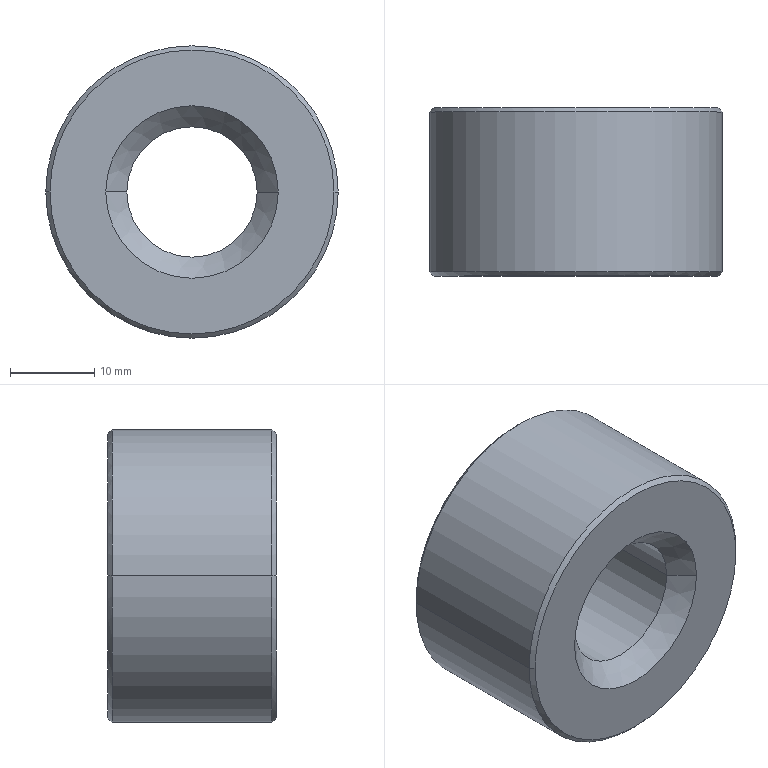Part | STEP file | CIHUAN_7_1 | 1 solid | 14 faces | box 34.75 x 20 x 34.75 mm | volume 14830 mm3 | cone 8 | cylinder 4 | plane 2 | commonest cylinder face diameters 15.5 x2 34.75 x2
STEP:
#1=CARTESIAN_POINT('',(0.,0.,0.));
#2=DIRECTION('',(0.,0.,1.));
#3=DIRECTION('',(1.,0.,0.));
#4=AXIS2_PLACEMENT_3D('',#1,#2,#3);
#5=CARTESIAN_POINT('',(16.875,0.,0.));
#6=VERTEX_POINT('',#5);
#7=CARTESIAN_POINT('',(0.,0.,-16.875));
#8=VERTEX_POINT('',#7);
#9=CARTESIAN_POINT('',(0.,0.,0.));
#10=DIRECTION('',(0.,1.,0.));
#11=DIRECTION('',(1.,0.,0.));
#12=AXIS2_PLACEMENT_3D('',#9,#10,#11);
#13=CIRCLE('',#12,16.875);
#14=EDGE_CURVE('',#6,#8,#13,.T.);
#15=ORIENTED_EDGE('',*,*,#14,.T.);
#16=CARTESIAN_POINT('',(-16.875,0.,0.));
#17=VERTEX_POINT('',#16);
#18=CARTESIAN_POINT('',(0.,0.,0.));
#19=DIRECTION('',(0.,1.,0.));
#20=DIRECTION('',(0.,0.,-1.));
#21=AXIS2_PLACEMENT_3D('',#18,#19,#20);
#22=CIRCLE('',#21,16.875);
#23=EDGE_CURVE('',#8,#17,#22,.T.);
#24=ORIENTED_EDGE('',*,*,#23,.T.);
#25=CARTESIAN_POINT('',(0.,0.,16.875));
#26=VERTEX_POINT('',#25);
#27=CARTESIAN_POINT('',(0.,0.,0.));
#28=DIRECTION('',(0.,1.,0.));
#29=DIRECTION('',(-1.,0.,0.));
#30=AXIS2_PLACEMENT_3D('',#27,#28,#29);
#31=CIRCLE('',#30,16.875);
#32=EDGE_CURVE('',#17,#26,#31,.T.);
#33=ORIENTED_EDGE('',*,*,#32,.T.);
#34=CARTESIAN_POINT('',(0.,0.,0.));
#35=DIRECTION('',(0.,1.,0.));
#36=DIRECTION('',(0.,0.,1.));
#37=AXIS2_PLACEMENT_3D('',#34,#35,#36);
#38=CIRCLE('',#37,16.875);
#39=EDGE_CURVE('',#26,#6,#38,.T.);
#40=ORIENTED_EDGE('',*,*,#39,.T.);
#41=EDGE_LOOP('',(#15,#24,#33,#40));
#42=FACE_OUTER_BOUND('',#41,.F.);
#43=CARTESIAN_POINT('',(-10.25,0.,0.));
#44=VERTEX_POINT('',#43);
#45=CARTESIAN_POINT('',(0.,0.,-10.25));
#46=VERTEX_POINT('',#45);
#47=CARTESIAN_POINT('',(0.,0.,0.));
#48=DIRECTION('',(0.,-1.,0.));
#49=DIRECTION('',(-1.,0.,0.));
#50=AXIS2_PLACEMENT_3D('',#47,#48,#49);
#51=CIRCLE('',#50,10.25);
#52=EDGE_CURVE('',#44,#46,#51,.T.);
#53=ORIENTED_EDGE('',*,*,#52,.T.);
#54=CARTESIAN_POINT('',(10.25,0.,0.));
#55=VERTEX_POINT('',#54);
#56=CARTESIAN_POINT('',(0.,0.,0.));
#57=DIRECTION('',(0.,-1.,0.));
#58=DIRECTION('',(0.,0.,-1.));
#59=AXIS2_PLACEMENT_3D('',#56,#57,#58);
#60=CIRCLE('',#59,10.25);
#61=EDGE_CURVE('',#46,#55,#60,.T.);
#62=ORIENTED_EDGE('',*,*,#61,.T.);
#63=CARTESIAN_POINT('',(0.,0.,10.25));
#64=VERTEX_POINT('',#63);
#65=CARTESIAN_POINT('',(0.,0.,0.));
#66=DIRECTION('',(0.,-1.,0.));
#67=DIRECTION('',(1.,0.,0.));
#68=AXIS2_PLACEMENT_3D('',#65,#66,#67);
#69=CIRCLE('',#68,10.25);
#70=EDGE_CURVE('',#55,#64,#69,.T.);
#71=ORIENTED_EDGE('',*,*,#70,.T.);
#72=CARTESIAN_POINT('',(0.,0.,0.));
#73=DIRECTION('',(0.,-1.,0.));
#74=DIRECTION('',(0.,0.,1.));
#75=AXIS2_PLACEMENT_3D('',#72,#73,#74);
#76=CIRCLE('',#75,10.25);
#77=EDGE_CURVE('',#64,#44,#76,.T.);
#78=ORIENTED_EDGE('',*,*,#77,.T.);
#79=EDGE_LOOP('',(#53,#62,#71,#78));
#80=FACE_BOUND('',#79,.F.);
#81=CARTESIAN_POINT('',(0.,0.,0.));
#82=DIRECTION('',(0.,1.,0.));
#83=DIRECTION('',(1.,0.,0.));
#84=AXIS2_PLACEMENT_3D('',#81,#82,#83);
#85=PLANE('',#84);
#86=ADVANCED_FACE('',(#42,#80),#85,.F.);
#87=ORIENTED_EDGE('',*,*,#23,.F.);
#88=ORIENTED_EDGE('',*,*,#14,.F.);
#89=CARTESIAN_POINT('',(17.375,0.5,-0.000000001));
#90=VERTEX_POINT('',#89);
#91=CARTESIAN_POINT('',(16.875,0.,-0.000000001));
#92=DIRECTION('',(0.7071,0.7071,0.));
#93=VECTOR('',#92,0.7071);
#94=LINE('',#91,#93);
#95=EDGE_CURVE('',#6,#90,#94,.T.);
#96=ORIENTED_EDGE('',*,*,#95,.T.);
#97=CARTESIAN_POINT('',(0.,0.5,-17.375));
#98=VERTEX_POINT('',#97);
#99=CARTESIAN_POINT('',(0.,0.5,0.));
#100=DIRECTION('',(0.,1.,0.));
#101=DIRECTION('',(1.,0.,0.));
#102=AXIS2_PLACEMENT_3D('',#99,#100,#101);
#103=CIRCLE('',#102,17.375);
#104=EDGE_CURVE('',#90,#98,#103,.T.);
#105=ORIENTED_EDGE('',*,*,#104,.T.);
#106=CARTESIAN_POINT('',(-17.375,0.5,0.000000002));
#107=VERTEX_POINT('',#106);
#108=CARTESIAN_POINT('',(0.,0.5,0.));
#109=DIRECTION('',(0.,1.,0.));
#110=DIRECTION('',(0.,0.,-1.));
#111=AXIS2_PLACEMENT_3D('',#108,#109,#110);
#112=CIRCLE('',#111,17.375);
#113=EDGE_CURVE('',#98,#107,#112,.T.);
#114=ORIENTED_EDGE('',*,*,#113,.T.);
#115=CARTESIAN_POINT('',(-16.875,0.,0.000000001));
#116=DIRECTION('',(-0.7071,0.7071,0.000000001));
#117=VECTOR('',#116,0.7071);
#118=LINE('',#115,#117);
#119=EDGE_CURVE('',#17,#107,#118,.T.);
#120=ORIENTED_EDGE('',*,*,#119,.F.);
#121=EDGE_LOOP('',(#87,#88,#96,#105,#114,#120));
#122=FACE_OUTER_BOUND('',#121,.F.);
#123=CARTESIAN_POINT('',(0.,0.25,0.));
#124=DIRECTION('',(0.,1.,0.));
#125=DIRECTION('',(0.,0.,-1.));
#126=AXIS2_PLACEMENT_3D('',#123,#124,#125);
#127=CONICAL_SURFACE('',#126,17.125,45.);
#128=ADVANCED_FACE('',(#122),#127,.T.);
#129=ORIENTED_EDGE('',*,*,#39,.F.);
#130=ORIENTED_EDGE('',*,*,#32,.F.);
#131=ORIENTED_EDGE('',*,*,#119,.T.);
#132=CARTESIAN_POINT('',(0.,0.5,17.375));
#133=VERTEX_POINT('',#132);
#134=CARTESIAN_POINT('',(0.,0.5,0.));
#135=DIRECTION('',(0.,1.,0.));
#136=DIRECTION('',(-1.,0.,0.));
#137=AXIS2_PLACEMENT_3D('',#134,#135,#136);
#138=CIRCLE('',#137,17.375);
#139=EDGE_CURVE('',#107,#133,#138,.T.);
#140=ORIENTED_EDGE('',*,*,#139,.T.);
#141=CARTESIAN_POINT('',(0.,0.5,0.));
#142=DIRECTION('',(0.,1.,0.));
#143=DIRECTION('',(0.,0.,1.));
#144=AXIS2_PLACEMENT_3D('',#141,#142,#143);
#145=CIRCLE('',#144,17.375);
#146=EDGE_CURVE('',#133,#90,#145,.T.);
#147=ORIENTED_EDGE('',*,*,#146,.T.);
#148=ORIENTED_EDGE('',*,*,#95,.F.);
#149=EDGE_LOOP('',(#129,#130,#131,#140,#147,#148));
#150=FACE_OUTER_BOUND('',#149,.F.);
#151=CARTESIAN_POINT('',(0.,0.25,0.));
#152=DIRECTION('',(0.,1.,0.));
#153=DIRECTION('',(0.,0.,-1.));
#154=AXIS2_PLACEMENT_3D('',#151,#152,#153);
#155=CONICAL_SURFACE('',#154,17.125,45.);
#156=ADVANCED_FACE('',(#150),#155,.T.);
#157=CARTESIAN_POINT('',(0.,19.5,17.375));
#158=VERTEX_POINT('',#157);
#159=CARTESIAN_POINT('',(-17.375,19.5,0.000000002));
#160=VERTEX_POINT('',#159);
#161=CARTESIAN_POINT('',(0.,19.5,0.));
#162=DIRECTION('',(0.,-1.,0.));
#163=DIRECTION('',(0.,0.,1.));
#164=AXIS2_PLACEMENT_3D('',#161,#162,#163);
#165=CIRCLE('',#164,17.375);
#166=EDGE_CURVE('',#158,#160,#165,.T.);
#167=ORIENTED_EDGE('',*,*,#166,.F.);
#168=CARTESIAN_POINT('',(17.375,19.5,0.));
#169=VERTEX_POINT('',#168);
#170=CARTESIAN_POINT('',(0.,19.5,0.));
#171=DIRECTION('',(0.,-1.,0.));
#172=DIRECTION('',(1.,0.,0.));
#173=AXIS2_PLACEMENT_3D('',#170,#171,#172);
#174=CIRCLE('',#173,17.375);
#175=EDGE_CURVE('',#169,#158,#174,.T.);
#176=ORIENTED_EDGE('',*,*,#175,.F.);
#177=CARTESIAN_POINT('',(17.375,0.5,-0.000000001));
#178=DIRECTION('',(0.,1.,0.));
#179=VECTOR('',#178,19.);
#180=LINE('',#177,#179);
#181=EDGE_CURVE('',#90,#169,#180,.T.);
#182=ORIENTED_EDGE('',*,*,#181,.F.);
#183=ORIENTED_EDGE('',*,*,#146,.F.);
#184=ORIENTED_EDGE('',*,*,#139,.F.);
#185=CARTESIAN_POINT('',(-17.375,0.5,0.000000002));
#186=DIRECTION('',(0.,1.,0.));
#187=VECTOR('',#186,19.);
#188=LINE('',#185,#187);
#189=EDGE_CURVE('',#107,#160,#188,.T.);
#190=ORIENTED_EDGE('',*,*,#189,.T.);
#191=EDGE_LOOP('',(#167,#176,#182,#183,#184,#190));
#192=FACE_OUTER_BOUND('',#191,.F.);
#193=CARTESIAN_POINT('',(0.,0.,0.));
#194=DIRECTION('',(0.,1.,0.));
#195=DIRECTION('',(1.,0.,0.));
#196=AXIS2_PLACEMENT_3D('',#193,#194,#195);
#197=CYLINDRICAL_SURFACE('',#196,17.375);
#198=ADVANCED_FACE('',(#192),#197,.T.);
#199=CARTESIAN_POINT('',(0.,20.,16.875));
#200=VERTEX_POINT('',#199);
#201=CARTESIAN_POINT('',(-16.875,20.,0.));
#202=VERTEX_POINT('',#201);
#203=CARTESIAN_POINT('',(0.,20.,0.));
#204=DIRECTION('',(0.,-1.,0.));
#205=DIRECTION('',(0.,0.,1.));
#206=AXIS2_PLACEMENT_3D('',#203,#204,#205);
#207=CIRCLE('',#206,16.875);
#208=EDGE_CURVE('',#200,#202,#207,.T.);
#209=ORIENTED_EDGE('',*,*,#208,.F.);
#210=CARTESIAN_POINT('',(16.875,20.,0.));
#211=VERTEX_POINT('',#210);
#212=CARTESIAN_POINT('',(0.,20.,0.));
#213=DIRECTION('',(0.,-1.,0.));
#214=DIRECTION('',(1.,0.,0.));
#215=AXIS2_PLACEMENT_3D('',#212,#213,#214);
#216=CIRCLE('',#215,16.875);
#217=EDGE_CURVE('',#211,#200,#216,.T.);
#218=ORIENTED_EDGE('',*,*,#217,.F.);
#219=CARTESIAN_POINT('',(16.875,20.,-0.000000001));
#220=DIRECTION('',(0.7071,-0.7071,0.));
#221=VECTOR('',#220,0.7071);
#222=LINE('',#219,#221);
#223=EDGE_CURVE('',#211,#169,#222,.T.);
#224=ORIENTED_EDGE('',*,*,#223,.T.);
#225=ORIENTED_EDGE('',*,*,#175,.T.);
#226=ORIENTED_EDGE('',*,*,#166,.T.);
#227=CARTESIAN_POINT('',(-16.875,20.,0.000000001));
#228=DIRECTION('',(-0.7071,-0.7071,0.000000001));
#229=VECTOR('',#228,0.7071);
#230=LINE('',#227,#229);
#231=EDGE_CURVE('',#202,#160,#230,.T.);
#232=ORIENTED_EDGE('',*,*,#231,.F.);
#233=EDGE_LOOP('',(#209,#218,#224,#225,#226,#232));
#234=FACE_OUTER_BOUND('',#233,.F.);
#235=CARTESIAN_POINT('',(0.,19.75,0.));
#236=DIRECTION('',(0.,-1.,0.));
#237=DIRECTION('',(0.,0.,-1.));
#238=AXIS2_PLACEMENT_3D('',#235,#236,#237);
#239=CONICAL_SURFACE('',#238,17.125,45.);
#240=ADVANCED_FACE('',(#234),#239,.T.);
#241=CARTESIAN_POINT('',(0.,20.,-16.875));
#242=VERTEX_POINT('',#241);
#243=CARTESIAN_POINT('',(0.,20.,0.));
#244=DIRECTION('',(0.,-1.,0.));
#245=DIRECTION('',(-1.,0.,0.));
#246=AXIS2_PLACEMENT_3D('',#243,#244,#245);
#247=CIRCLE('',#246,16.875);
#248=EDGE_CURVE('',#202,#242,#247,.T.);
#249=ORIENTED_EDGE('',*,*,#248,.T.);
#250=CARTESIAN_POINT('',(0.,20.,0.));
#251=DIRECTION('',(0.,-1.,0.));
#252=DIRECTION('',(0.,0.,-1.));
#253=AXIS2_PLACEMENT_3D('',#250,#251,#252);
#254=CIRCLE('',#253,16.875);
#255=EDGE_CURVE('',#242,#211,#254,.T.);
#256=ORIENTED_EDGE('',*,*,#255,.T.);
#257=ORIENTED_EDGE('',*,*,#217,.T.);
#258=ORIENTED_EDGE('',*,*,#208,.T.);
#259=EDGE_LOOP('',(#249,#256,#257,#258));
#260=FACE_OUTER_BOUND('',#259,.F.);
#261=CARTESIAN_POINT('',(10.25,20.,0.));
#262=VERTEX_POINT('',#261);
#263=CARTESIAN_POINT('',(0.,20.,-10.25));
#264=VERTEX_POINT('',#263);
#265=CARTESIAN_POINT('',(0.,20.,0.));
#266=DIRECTION('',(0.,1.,0.));
#267=DIRECTION('',(1.,0.,0.));
#268=AXIS2_PLACEMENT_3D('',#265,#266,#267);
#269=CIRCLE('',#268,10.25);
#270=EDGE_CURVE('',#262,#264,#269,.T.);
#271=ORIENTED_EDGE('',*,*,#270,.T.);
#272=CARTESIAN_POINT('',(-10.25,20.,0.));
#273=VERTEX_POINT('',#272);
#274=CARTESIAN_POINT('',(0.,20.,0.));
#275=DIRECTION('',(0.,1.,0.));
#276=DIRECTION('',(0.,0.,-1.));
#277=AXIS2_PLACEMENT_3D('',#274,#275,#276);
#278=CIRCLE('',#277,10.25);
#279=EDGE_CURVE('',#264,#273,#278,.T.);
#280=ORIENTED_EDGE('',*,*,#279,.T.);
#281=CARTESIAN_POINT('',(0.,20.,10.25));
#282=VERTEX_POINT('',#281);
#283=CARTESIAN_POINT('',(0.,20.,0.));
#284=DIRECTION('',(0.,1.,0.));
#285=DIRECTION('',(-1.,0.,0.));
#286=AXIS2_PLACEMENT_3D('',#283,#284,#285);
#287=CIRCLE('',#286,10.25);
#288=EDGE_CURVE('',#273,#282,#287,.T.);
#289=ORIENTED_EDGE('',*,*,#288,.T.);
#290=CARTESIAN_POINT('',(0.,20.,0.));
#291=DIRECTION('',(0.,1.,0.));
#292=DIRECTION('',(0.,0.,1.));
#293=AXIS2_PLACEMENT_3D('',#290,#291,#292);
#294=CIRCLE('',#293,10.25);
#295=EDGE_CURVE('',#282,#262,#294,.T.);
#296=ORIENTED_EDGE('',*,*,#295,.T.);
#297=EDGE_LOOP('',(#271,#280,#289,#296));
#298=FACE_BOUND('',#297,.F.);
#299=CARTESIAN_POINT('',(0.,20.,0.));
#300=DIRECTION('',(0.,1.,0.));
#301=DIRECTION('',(1.,0.,0.));
#302=AXIS2_PLACEMENT_3D('',#299,#300,#301);
#303=PLANE('',#302);
#304=ADVANCED_FACE('',(#260,#298),#303,.T.);
#305=ORIENTED_EDGE('',*,*,#255,.F.);
#306=ORIENTED_EDGE('',*,*,#248,.F.);
#307=ORIENTED_EDGE('',*,*,#231,.T.);
#308=CARTESIAN_POINT('',(0.,19.5,-17.375));
#309=VERTEX_POINT('',#308);
#310=CARTESIAN_POINT('',(0.,19.5,0.));
#311=DIRECTION('',(0.,-1.,0.));
#312=DIRECTION('',(-1.,0.,0.));
#313=AXIS2_PLACEMENT_3D('',#310,#311,#312);
#314=CIRCLE('',#313,17.375);
#315=EDGE_CURVE('',#160,#309,#314,.T.);
#316=ORIENTED_EDGE('',*,*,#315,.T.);
#317=CARTESIAN_POINT('',(0.,19.5,0.));
#318=DIRECTION('',(0.,-1.,0.));
#319=DIRECTION('',(0.,0.,-1.));
#320=AXIS2_PLACEMENT_3D('',#317,#318,#319);
#321=CIRCLE('',#320,17.375);
#322=EDGE_CURVE('',#309,#169,#321,.T.);
#323=ORIENTED_EDGE('',*,*,#322,.T.);
#324=ORIENTED_EDGE('',*,*,#223,.F.);
#325=EDGE_LOOP('',(#305,#306,#307,#316,#323,#324));
#326=FACE_OUTER_BOUND('',#325,.F.);
#327=CARTESIAN_POINT('',(0.,19.75,0.));
#328=DIRECTION('',(0.,-1.,0.));
#329=DIRECTION('',(0.,0.,-1.));
#330=AXIS2_PLACEMENT_3D('',#327,#328,#329);
#331=CONICAL_SURFACE('',#330,17.125,45.);
#332=ADVANCED_FACE('',(#326),#331,.T.);
#333=ORIENTED_EDGE('',*,*,#322,.F.);
#334=ORIENTED_EDGE('',*,*,#315,.F.);
#335=ORIENTED_EDGE('',*,*,#189,.F.);
#336=ORIENTED_EDGE('',*,*,#113,.F.);
#337=ORIENTED_EDGE('',*,*,#104,.F.);
#338=ORIENTED_EDGE('',*,*,#181,.T.);
#339=EDGE_LOOP('',(#333,#334,#335,#336,#337,#338));
#340=FACE_OUTER_BOUND('',#339,.F.);
#341=CARTESIAN_POINT('',(0.,0.,0.));
#342=DIRECTION('',(0.,1.,0.));
#343=DIRECTION('',(1.,0.,0.));
#344=AXIS2_PLACEMENT_3D('',#341,#342,#343);
#345=CYLINDRICAL_SURFACE('',#344,17.375);
#346=ADVANCED_FACE('',(#340),#345,.T.);
#347=ORIENTED_EDGE('',*,*,#279,.F.);
#348=ORIENTED_EDGE('',*,*,#270,.F.);
#349=CARTESIAN_POINT('',(7.75,17.5,-0.000000001));
#350=VERTEX_POINT('',#349);
#351=CARTESIAN_POINT('',(10.25,20.,-0.000000002));
#352=DIRECTION('',(-0.7071,-0.7071,0.));
#353=VECTOR('',#352,3.536);
#354=LINE('',#351,#353);
#355=EDGE_CURVE('',#262,#350,#354,.T.);
#356=ORIENTED_EDGE('',*,*,#355,.T.);
#357=CARTESIAN_POINT('',(0.,17.5,-7.75));
#358=VERTEX_POINT('',#357);
#359=CARTESIAN_POINT('',(0.,17.5,0.));
#360=DIRECTION('',(0.,1.,0.));
#361=DIRECTION('',(1.,0.,0.));
#362=AXIS2_PLACEMENT_3D('',#359,#360,#361);
#363=CIRCLE('',#362,7.75);
#364=EDGE_CURVE('',#350,#358,#363,.T.);
#365=ORIENTED_EDGE('',*,*,#364,.T.);
#366=CARTESIAN_POINT('',(-7.75,17.5,0.000000003));
#367=VERTEX_POINT('',#366);
#368=CARTESIAN_POINT('',(0.,17.5,0.));
#369=DIRECTION('',(0.,1.,0.));
#370=DIRECTION('',(0.,0.,-1.));
#371=AXIS2_PLACEMENT_3D('',#368,#369,#370);
#372=CIRCLE('',#371,7.75);
#373=EDGE_CURVE('',#358,#367,#372,.T.);
#374=ORIENTED_EDGE('',*,*,#373,.T.);
#375=CARTESIAN_POINT('',(-10.25,20.,0.000000002));
#376=DIRECTION('',(0.7071,-0.7071,0.));
#377=VECTOR('',#376,3.536);
#378=LINE('',#375,#377);
#379=EDGE_CURVE('',#273,#367,#378,.T.);
#380=ORIENTED_EDGE('',*,*,#379,.F.);
#381=EDGE_LOOP('',(#347,#348,#356,#365,#374,#380));
#382=FACE_OUTER_BOUND('',#381,.F.);
#383=CARTESIAN_POINT('',(0.,18.75,0.));
#384=DIRECTION('',(0.,1.,0.));
#385=DIRECTION('',(0.,0.,-1.));
#386=AXIS2_PLACEMENT_3D('',#383,#384,#385);
#387=CONICAL_SURFACE('',#386,9.,45.);
#388=ADVANCED_FACE('',(#382),#387,.F.);
#389=ORIENTED_EDGE('',*,*,#295,.F.);
#390=ORIENTED_EDGE('',*,*,#288,.F.);
#391=ORIENTED_EDGE('',*,*,#379,.T.);
#392=CARTESIAN_POINT('',(0.,17.5,7.75));
#393=VERTEX_POINT('',#392);
#394=CARTESIAN_POINT('',(0.,17.5,0.));
#395=DIRECTION('',(0.,1.,0.));
#396=DIRECTION('',(-1.,0.,0.));
#397=AXIS2_PLACEMENT_3D('',#394,#395,#396);
#398=CIRCLE('',#397,7.75);
#399=EDGE_CURVE('',#367,#393,#398,.T.);
#400=ORIENTED_EDGE('',*,*,#399,.T.);
#401=CARTESIAN_POINT('',(0.,17.5,0.));
#402=DIRECTION('',(0.,1.,0.));
#403=DIRECTION('',(0.,0.,1.));
#404=AXIS2_PLACEMENT_3D('',#401,#402,#403);
#405=CIRCLE('',#404,7.75);
#406=EDGE_CURVE('',#393,#350,#405,.T.);
#407=ORIENTED_EDGE('',*,*,#406,.T.);
#408=ORIENTED_EDGE('',*,*,#355,.F.);
#409=EDGE_LOOP('',(#389,#390,#391,#400,#407,#408));
#410=FACE_OUTER_BOUND('',#409,.F.);
#411=CARTESIAN_POINT('',(0.,18.75,0.));
#412=DIRECTION('',(0.,1.,0.));
#413=DIRECTION('',(0.,0.,-1.));
#414=AXIS2_PLACEMENT_3D('',#411,#412,#413);
#415=CONICAL_SURFACE('',#414,9.,45.);
#416=ADVANCED_FACE('',(#410),#415,.F.);
#417=ORIENTED_EDGE('',*,*,#406,.F.);
#418=ORIENTED_EDGE('',*,*,#399,.F.);
#419=CARTESIAN_POINT('',(-7.75,2.5,0.000000003));
#420=VERTEX_POINT('',#419);
#421=CARTESIAN_POINT('',(-7.75,2.5,0.000000003));
#422=DIRECTION('',(0.,1.,0.));
#423=VECTOR('',#422,15.);
#424=LINE('',#421,#423);
#425=EDGE_CURVE('',#420,#367,#424,.T.);
#426=ORIENTED_EDGE('',*,*,#425,.F.);
#427=CARTESIAN_POINT('',(0.,2.5,7.75));
#428=VERTEX_POINT('',#427);
#429=CARTESIAN_POINT('',(0.,2.5,0.));
#430=DIRECTION('',(0.,-1.,0.));
#431=DIRECTION('',(0.,0.,1.));
#432=AXIS2_PLACEMENT_3D('',#429,#430,#431);
#433=CIRCLE('',#432,7.75);
#434=EDGE_CURVE('',#428,#420,#433,.T.);
#435=ORIENTED_EDGE('',*,*,#434,.F.);
#436=CARTESIAN_POINT('',(7.75,2.5,0.));
#437=VERTEX_POINT('',#436);
#438=CARTESIAN_POINT('',(0.,2.5,0.));
#439=DIRECTION('',(0.,-1.,0.));
#440=DIRECTION('',(1.,0.,0.));
#441=AXIS2_PLACEMENT_3D('',#438,#439,#440);
#442=CIRCLE('',#441,7.75);
#443=EDGE_CURVE('',#437,#428,#442,.T.);
#444=ORIENTED_EDGE('',*,*,#443,.F.);
#445=CARTESIAN_POINT('',(7.75,2.5,-0.000000001));
#446=DIRECTION('',(0.,1.,0.));
#447=VECTOR('',#446,15.);
#448=LINE('',#445,#447);
#449=EDGE_CURVE('',#437,#350,#448,.T.);
#450=ORIENTED_EDGE('',*,*,#449,.T.);
#451=EDGE_LOOP('',(#417,#418,#426,#435,#444,#450));
#452=FACE_OUTER_BOUND('',#451,.F.);
#453=CARTESIAN_POINT('',(0.,0.,0.));
#454=DIRECTION('',(0.,1.,0.));
#455=DIRECTION('',(1.,0.,0.));
#456=AXIS2_PLACEMENT_3D('',#453,#454,#455);
#457=CYLINDRICAL_SURFACE('',#456,7.75);
#458=ADVANCED_FACE('',(#452),#457,.F.);
#459=ORIENTED_EDGE('',*,*,#373,.F.);
#460=ORIENTED_EDGE('',*,*,#364,.F.);
#461=ORIENTED_EDGE('',*,*,#449,.F.);
#462=CARTESIAN_POINT('',(0.,2.5,-7.75));
#463=VERTEX_POINT('',#462);
#464=CARTESIAN_POINT('',(0.,2.5,0.));
#465=DIRECTION('',(0.,-1.,0.));
#466=DIRECTION('',(0.,0.,-1.));
#467=AXIS2_PLACEMENT_3D('',#464,#465,#466);
#468=CIRCLE('',#467,7.75);
#469=EDGE_CURVE('',#463,#437,#468,.T.);
#470=ORIENTED_EDGE('',*,*,#469,.F.);
#471=CARTESIAN_POINT('',(0.,2.5,0.));
#472=DIRECTION('',(0.,-1.,0.));
#473=DIRECTION('',(-1.,0.,0.));
#474=AXIS2_PLACEMENT_3D('',#471,#472,#473);
#475=CIRCLE('',#474,7.75);
#476=EDGE_CURVE('',#420,#463,#475,.T.);
#477=ORIENTED_EDGE('',*,*,#476,.F.);
#478=ORIENTED_EDGE('',*,*,#425,.T.);
#479=EDGE_LOOP('',(#459,#460,#461,#470,#477,#478));
#480=FACE_OUTER_BOUND('',#479,.F.);
#481=CARTESIAN_POINT('',(0.,0.,0.));
#482=DIRECTION('',(0.,1.,0.));
#483=DIRECTION('',(1.,0.,0.));
#484=AXIS2_PLACEMENT_3D('',#481,#482,#483);
#485=CYLINDRICAL_SURFACE('',#484,7.75);
#486=ADVANCED_FACE('',(#480),#485,.F.);
#487=ORIENTED_EDGE('',*,*,#61,.F.);
#488=ORIENTED_EDGE('',*,*,#52,.F.);
#489=CARTESIAN_POINT('',(-10.25,0.,0.000000002));
#490=DIRECTION('',(0.7071,0.7071,0.));
#491=VECTOR('',#490,3.536);
#492=LINE('',#489,#491);
#493=EDGE_CURVE('',#44,#420,#492,.T.);
#494=ORIENTED_EDGE('',*,*,#493,.T.);
#495=ORIENTED_EDGE('',*,*,#476,.T.);
#496=ORIENTED_EDGE('',*,*,#469,.T.);
#497=CARTESIAN_POINT('',(10.25,0.,-0.000000002));
#498=DIRECTION('',(-0.7071,0.7071,0.));
#499=VECTOR('',#498,3.536);
#500=LINE('',#497,#499);
#501=EDGE_CURVE('',#55,#437,#500,.T.);
#502=ORIENTED_EDGE('',*,*,#501,.F.);
#503=EDGE_LOOP('',(#487,#488,#494,#495,#496,#502));
#504=FACE_OUTER_BOUND('',#503,.F.);
#505=CARTESIAN_POINT('',(0.,1.25,0.));
#506=DIRECTION('',(0.,-1.,0.));
#507=DIRECTION('',(0.,0.,-1.));
#508=AXIS2_PLACEMENT_3D('',#505,#506,#507);
#509=CONICAL_SURFACE('',#508,9.,45.);
#510=ADVANCED_FACE('',(#504),#509,.F.);
#511=ORIENTED_EDGE('',*,*,#77,.F.);
#512=ORIENTED_EDGE('',*,*,#70,.F.);
#513=ORIENTED_EDGE('',*,*,#501,.T.);
#514=ORIENTED_EDGE('',*,*,#443,.T.);
#515=ORIENTED_EDGE('',*,*,#434,.T.);
#516=ORIENTED_EDGE('',*,*,#493,.F.);
#517=EDGE_LOOP('',(#511,#512,#513,#514,#515,#516));
#518=FACE_OUTER_BOUND('',#517,.F.);
#519=CARTESIAN_POINT('',(0.,1.25,0.));
#520=DIRECTION('',(0.,-1.,0.));
#521=DIRECTION('',(0.,0.,-1.));
#522=AXIS2_PLACEMENT_3D('',#519,#520,#521);
#523=CONICAL_SURFACE('',#522,9.,45.);
#524=ADVANCED_FACE('',(#518),#523,.F.);
#525=CLOSED_SHELL('',(#86,#128,#156,#198,#240,#304,#332,#346,#388,#416,#458,#486,#510,#524));
#526=MANIFOLD_SOLID_BREP('',#525);
#527=(LENGTH_UNIT()NAMED_UNIT(*)SI_UNIT(.MILLI.,.METRE.));
#528=UNCERTAINTY_MEASURE_WITH_UNIT(LENGTH_MEASURE(0.005306),#527,'','');
#529=(NAMED_UNIT(*)PLANE_ANGLE_UNIT()SI_UNIT($,.RADIAN.));
#530=PLANE_ANGLE_MEASURE_WITH_UNIT(PLANE_ANGLE_MEASURE(0.01745),#529);
#531=(CONVERSION_BASED_UNIT('DEGREE',#530)NAMED_UNIT(*)PLANE_ANGLE_UNIT());
#532=(NAMED_UNIT(*)SI_UNIT($,.STERADIAN.)SOLID_ANGLE_UNIT());
#533=(GEOMETRIC_REPRESENTATION_CONTEXT(3)GLOBAL_UNCERTAINTY_ASSIGNED_CONTEXT((#528))GLOBAL_UNIT_ASSIGNED_CONTEXT((#527,#531,#532))REPRESENTATION_CONTEXT('',''));
#534=ADVANCED_BREP_SHAPE_REPRESENTATION('',(#4,#526),#533);